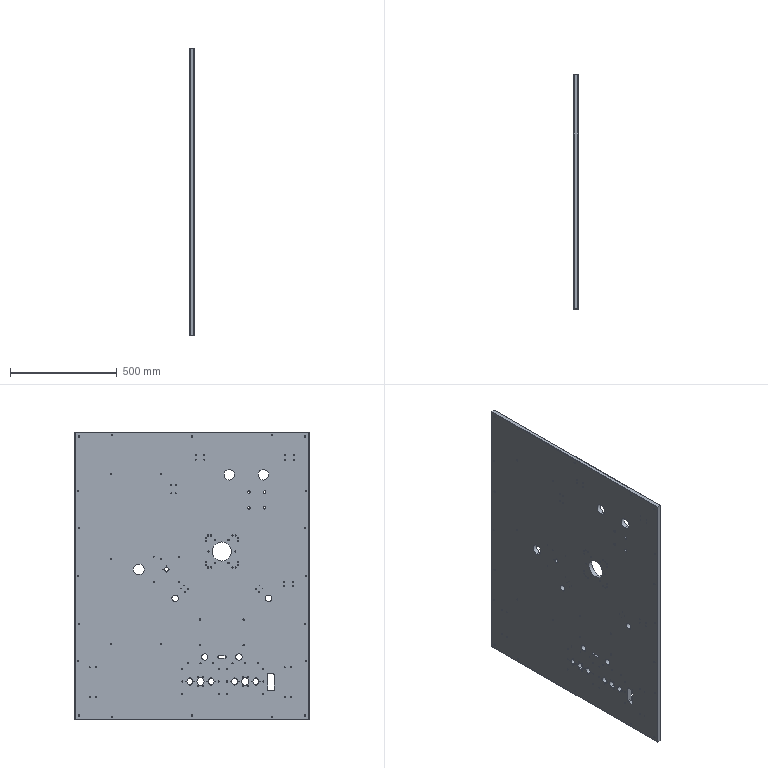Part | STEP file | 01-07 Base plate | 1 solid | 422 faces | box 20 x 1100 x 1350 mm | volume 29158066 mm3 | cylinder 364 | plane 58 | commonest cylinder face diameters 5 x96 5.5 x68 3.3 x56 10 x34 8.5 x20 15 x20